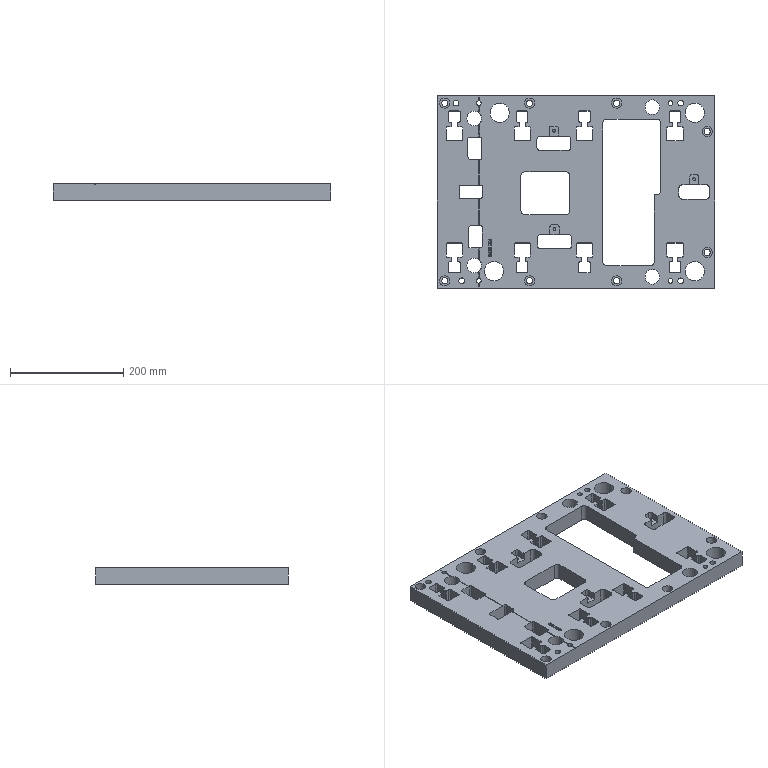Part | NX | features LIN_SOLID_COLOR 2 | 1 solid | 472 faces | box 490 x 340 x 30 mm | volume 3303514 mm3 | plane 263 | cylinder 176 | spline 30 | cone 3 | commonest cylinder face diameters 4 x48 4.04 x32 1 x16 10.04 x12 11 x11 5 x9